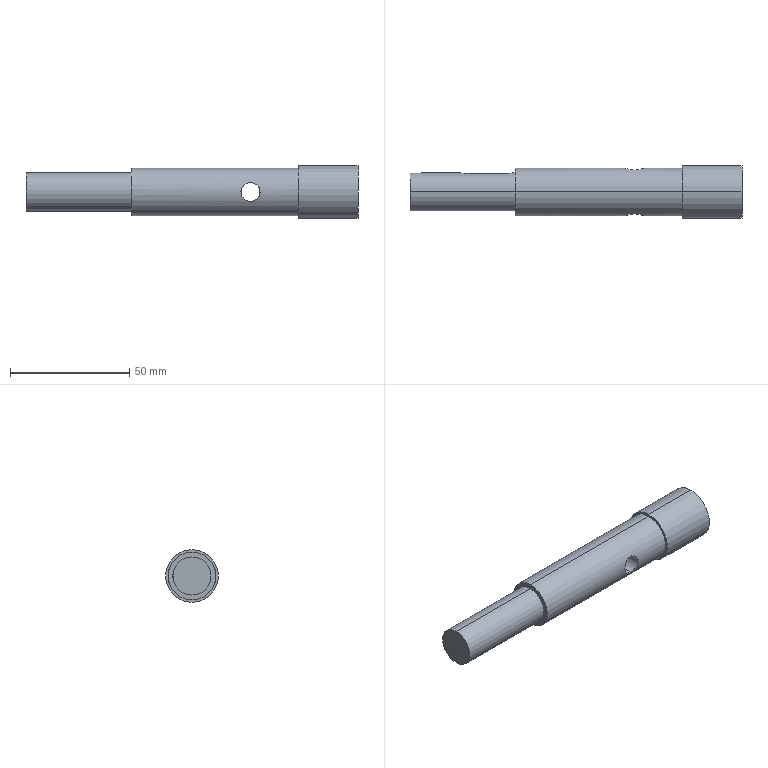Part | SolidWorks | features ICE 2, Revolution 1 | 1 solid | 20 faces | box 139 x 22 x 22 mm | volume 37145 mm3 | cylinder 13 | plane 7 | commonest cylinder face diameters 8 x5 4 x2 16 x2 20 x2 22 x2
STEP:
#1=CARTESIAN_POINT('',(94.,-9.165,-4.));
#2=VERTEX_POINT('',#1);
#3=CARTESIAN_POINT('',(94.,-9.165,4.));
#4=VERTEX_POINT('',#3);
#5=CARTESIAN_POINT('',(94.,-9.165,-4.));
#6=CARTESIAN_POINT('',(93.737,-9.165,-4.));
#7=CARTESIAN_POINT('',(93.471,-9.177,-3.974));
#8=CARTESIAN_POINT('',(92.952,-9.221,-3.869));
#9=CARTESIAN_POINT('',(92.702,-9.254,-3.793));
#10=CARTESIAN_POINT('',(92.219,-9.334,-3.591));
#11=CARTESIAN_POINT('',(91.987,-9.381,-3.466));
#12=CARTESIAN_POINT('',(91.557,-9.483,-3.178));
#13=CARTESIAN_POINT('',(91.356,-9.537,-3.013));
#14=CARTESIAN_POINT('',(90.987,-9.646,-2.644));
#15=CARTESIAN_POINT('',(90.823,-9.699,-2.444));
#16=CARTESIAN_POINT('',(90.535,-9.797,-2.015));
#17=CARTESIAN_POINT('',(90.409,-9.843,-1.782));
#18=CARTESIAN_POINT('',(90.208,-9.918,-1.299));
#19=CARTESIAN_POINT('',(90.131,-9.948,-1.049));
#20=CARTESIAN_POINT('',(90.027,-9.989,-0.5334));
#21=CARTESIAN_POINT('',(90.,-10.,-0.2654));
#22=CARTESIAN_POINT('',(90.,-10.,0.2618));
#23=CARTESIAN_POINT('',(90.026,-9.99,0.5238));
#24=CARTESIAN_POINT('',(90.13,-9.949,1.045));
#25=CARTESIAN_POINT('',(90.207,-9.919,1.297));
#26=CARTESIAN_POINT('',(90.408,-9.843,1.779));
#27=CARTESIAN_POINT('',(90.533,-9.798,2.012));
#28=CARTESIAN_POINT('',(90.823,-9.699,2.444));
#29=CARTESIAN_POINT('',(90.987,-9.646,2.644));
#30=CARTESIAN_POINT('',(91.354,-9.538,3.011));
#31=CARTESIAN_POINT('',(91.557,-9.483,3.177));
#32=CARTESIAN_POINT('',(91.986,-9.382,3.465));
#33=CARTESIAN_POINT('',(92.214,-9.335,3.589));
#34=CARTESIAN_POINT('',(92.7,-9.254,3.792));
#35=CARTESIAN_POINT('',(92.952,-9.221,3.869));
#36=CARTESIAN_POINT('',(93.467,-9.177,3.973));
#37=CARTESIAN_POINT('',(93.733,-9.165,4.));
#38=CARTESIAN_POINT('',(94.,-9.165,4.));
#39=B_SPLINE_CURVE_WITH_KNOTS('',3,(#5,#6,#7,#8,#9,#10,#11,#12,#13,#14,#15,#16,#17,#18,#19,#20,#21,#22,#23,#24,#25,#26,#27,#28,#29,#30,#31,#32,#33,#34,#35,#36,#37,#38),.UNSPECIFIED.,.F.,.F.,(4,2,2,2,2,2,2,2,2,2,2,2,2,2,2,2,4),(0.01264,0.01343,0.01422,0.01501,0.0158,0.01658,0.01737,0.01816,0.01895,0.01974,0.02053,0.02132,0.02211,0.0229,0.02369,0.02448,0.02527),.UNSPECIFIED.);
#40=EDGE_CURVE('',#2,#4,#39,.T.);
#41=ORIENTED_EDGE('',*,*,#40,.F.);
#42=CARTESIAN_POINT('',(94.,0.,-4.));
#43=VERTEX_POINT('',#42);
#44=CARTESIAN_POINT('',(94.,-11.,-4.));
#45=DIRECTION('',(0.,1.,0.));
#46=VECTOR('',#45,1000.);
#47=LINE('',#44,#46);
#48=EDGE_CURVE('',#2,#43,#47,.T.);
#49=ORIENTED_EDGE('',*,*,#48,.T.);
#50=CARTESIAN_POINT('',(94.,9.165,-4.));
#51=VERTEX_POINT('',#50);
#52=CARTESIAN_POINT('',(94.,-11.,-4.));
#53=DIRECTION('',(0.,1.,0.));
#54=VECTOR('',#53,1000.);
#55=LINE('',#52,#54);
#56=EDGE_CURVE('',#43,#51,#55,.T.);
#57=ORIENTED_EDGE('',*,*,#56,.T.);
#58=CARTESIAN_POINT('',(94.,9.165,4.));
#59=VERTEX_POINT('',#58);
#60=CARTESIAN_POINT('',(94.,9.165,4.));
#61=CARTESIAN_POINT('',(93.733,9.165,4.));
#62=CARTESIAN_POINT('',(93.47,9.177,3.973));
#63=CARTESIAN_POINT('',(92.955,9.221,3.87));
#64=CARTESIAN_POINT('',(92.7,9.254,3.792));
#65=CARTESIAN_POINT('',(92.217,9.334,3.59));
#66=CARTESIAN_POINT('',(91.989,9.381,3.467));
#67=CARTESIAN_POINT('',(91.556,9.483,3.177));
#68=CARTESIAN_POINT('',(91.354,9.538,3.011));
#69=CARTESIAN_POINT('',(90.989,9.646,2.646));
#70=CARTESIAN_POINT('',(90.824,9.699,2.445));
#71=CARTESIAN_POINT('',(90.532,9.798,2.01));
#72=CARTESIAN_POINT('',(90.409,9.843,1.781));
#73=CARTESIAN_POINT('',(90.208,9.918,1.301));
#74=CARTESIAN_POINT('',(90.13,9.949,1.046));
#75=CARTESIAN_POINT('',(90.026,9.989,0.5279));
#76=CARTESIAN_POINT('',(90.,10.,0.2663));
#77=CARTESIAN_POINT('',(90.,10.,-0.2622));
#78=CARTESIAN_POINT('',(90.027,9.989,-0.5302));
#79=CARTESIAN_POINT('',(90.13,9.949,-1.046));
#80=CARTESIAN_POINT('',(90.207,9.919,-1.297));
#81=CARTESIAN_POINT('',(90.411,9.842,-1.785));
#82=CARTESIAN_POINT('',(90.534,9.798,-2.014));
#83=CARTESIAN_POINT('',(90.824,9.699,-2.445));
#84=CARTESIAN_POINT('',(90.991,9.645,-2.648));
#85=CARTESIAN_POINT('',(91.358,9.537,-3.014));
#86=CARTESIAN_POINT('',(91.557,9.483,-3.178));
#87=CARTESIAN_POINT('',(91.989,9.381,-3.467));
#88=CARTESIAN_POINT('',(92.222,9.333,-3.592));
#89=CARTESIAN_POINT('',(92.702,9.254,-3.792));
#90=CARTESIAN_POINT('',(92.952,9.221,-3.869));
#91=CARTESIAN_POINT('',(93.473,9.177,-3.974));
#92=CARTESIAN_POINT('',(93.737,9.165,-4.));
#93=CARTESIAN_POINT('',(94.,9.165,-4.));
#94=B_SPLINE_CURVE_WITH_KNOTS('',3,(#60,#61,#62,#63,#64,#65,#66,#67,#68,#69,#70,#71,#72,#73,#74,#75,#76,#77,#78,#79,#80,#81,#82,#83,#84,#85,#86,#87,#88,#89,#90,#91,#92,#93),.UNSPECIFIED.,.F.,.F.,(4,2,2,2,2,2,2,2,2,2,2,2,2,2,2,2,4),(0.,0.0007899,0.00158,0.00237,0.00316,0.00395,0.00474,0.00553,0.006319,0.007109,0.007899,0.008689,0.009479,0.01027,0.01106,0.01185,0.01264),.UNSPECIFIED.);
#95=EDGE_CURVE('',#59,#51,#94,.T.);
#96=ORIENTED_EDGE('',*,*,#95,.F.);
#97=CARTESIAN_POINT('',(94.,0.,4.));
#98=VERTEX_POINT('',#97);
#99=CARTESIAN_POINT('',(94.,-11.,4.));
#100=DIRECTION('',(0.,1.,0.));
#101=VECTOR('',#100,1000.);
#102=LINE('',#99,#101);
#103=EDGE_CURVE('',#98,#59,#102,.T.);
#104=ORIENTED_EDGE('',*,*,#103,.F.);
#105=CARTESIAN_POINT('',(94.,-11.,4.));
#106=DIRECTION('',(0.,1.,0.));
#107=VECTOR('',#106,1000.);
#108=LINE('',#105,#107);
#109=EDGE_CURVE('',#4,#98,#108,.T.);
#110=ORIENTED_EDGE('',*,*,#109,.F.);
#111=EDGE_LOOP('',(#41,#49,#57,#96,#104,#110));
#112=FACE_OUTER_BOUND('',#111,.T.);
#113=CARTESIAN_POINT('',(94.,-11.,0.));
#114=DIRECTION('',(0.,1.,0.));
#115=DIRECTION('',(0.,0.,1.));
#116=AXIS2_PLACEMENT_3D('',#113,#114,#115);
#117=CYLINDRICAL_SURFACE('',#116,4.);
#118=ADVANCED_FACE('',(#112),#117,.F.);
#119=ORIENTED_EDGE('',*,*,#48,.F.);
#120=CARTESIAN_POINT('',(94.,-9.165,4.));
#121=CARTESIAN_POINT('',(94.267,-9.165,4.));
#122=CARTESIAN_POINT('',(94.53,-9.177,3.973));
#123=CARTESIAN_POINT('',(95.045,-9.221,3.87));
#124=CARTESIAN_POINT('',(95.3,-9.254,3.792));
#125=CARTESIAN_POINT('',(95.783,-9.334,3.59));
#126=CARTESIAN_POINT('',(96.011,-9.381,3.467));
#127=CARTESIAN_POINT('',(96.444,-9.483,3.177));
#128=CARTESIAN_POINT('',(96.646,-9.538,3.011));
#129=CARTESIAN_POINT('',(97.011,-9.646,2.646));
#130=CARTESIAN_POINT('',(97.176,-9.699,2.445));
#131=CARTESIAN_POINT('',(97.468,-9.798,2.01));
#132=CARTESIAN_POINT('',(97.591,-9.843,1.781));
#133=CARTESIAN_POINT('',(97.792,-9.918,1.301));
#134=CARTESIAN_POINT('',(97.87,-9.949,1.046));
#135=CARTESIAN_POINT('',(97.974,-9.989,0.5279));
#136=CARTESIAN_POINT('',(98.,-10.,0.2663));
#137=CARTESIAN_POINT('',(98.,-10.,-0.2622));
#138=CARTESIAN_POINT('',(97.973,-9.989,-0.5302));
#139=CARTESIAN_POINT('',(97.87,-9.949,-1.046));
#140=CARTESIAN_POINT('',(97.793,-9.919,-1.297));
#141=CARTESIAN_POINT('',(97.589,-9.842,-1.785));
#142=CARTESIAN_POINT('',(97.466,-9.798,-2.014));
#143=CARTESIAN_POINT('',(97.176,-9.699,-2.445));
#144=CARTESIAN_POINT('',(97.009,-9.645,-2.648));
#145=CARTESIAN_POINT('',(96.642,-9.537,-3.014));
#146=CARTESIAN_POINT('',(96.443,-9.483,-3.178));
#147=CARTESIAN_POINT('',(96.011,-9.381,-3.467));
#148=CARTESIAN_POINT('',(95.778,-9.333,-3.592));
#149=CARTESIAN_POINT('',(95.298,-9.254,-3.792));
#150=CARTESIAN_POINT('',(95.048,-9.221,-3.869));
#151=CARTESIAN_POINT('',(94.527,-9.177,-3.974));
#152=CARTESIAN_POINT('',(94.263,-9.165,-4.));
#153=CARTESIAN_POINT('',(94.,-9.165,-4.));
#154=B_SPLINE_CURVE_WITH_KNOTS('',3,(#120,#121,#122,#123,#124,#125,#126,#127,#128,#129,#130,#131,#132,#133,#134,#135,#136,#137,#138,#139,#140,#141,#142,#143,#144,#145,#146,#147,#148,#149,#150,#151,#152,#153),.UNSPECIFIED.,.F.,.F.,(4,2,2,2,2,2,2,2,2,2,2,2,2,2,2,2,4),(0.,0.0007899,0.00158,0.00237,0.00316,0.00395,0.00474,0.00553,0.006319,0.007109,0.007899,0.008689,0.009479,0.01027,0.01106,0.01185,0.01264),.UNSPECIFIED.);
#155=EDGE_CURVE('',#4,#2,#154,.T.);
#156=ORIENTED_EDGE('',*,*,#155,.F.);
#157=ORIENTED_EDGE('',*,*,#109,.T.);
#158=CARTESIAN_POINT('',(94.,0.,-4.));
#159=CARTESIAN_POINT('',(102.,-8.,-4.));
#160=CARTESIAN_POINT('',(102.,-8.,4.));
#161=CARTESIAN_POINT('',(94.,0.,4.));
#162=(BOUNDED_CURVE()B_SPLINE_CURVE(3,(#158,#159,#160,#161),.UNSPECIFIED.,.F.,.T.)B_SPLINE_CURVE_WITH_KNOTS((4,4),(1.571,4.712),.UNSPECIFIED.)CURVE()GEOMETRIC_REPRESENTATION_ITEM()RATIONAL_B_SPLINE_CURVE((1.,0.3333,0.3333,1.))REPRESENTATION_ITEM(''));
#163=EDGE_CURVE('',#43,#98,#162,.T.);
#164=ORIENTED_EDGE('',*,*,#163,.F.);
#165=EDGE_LOOP('',(#119,#156,#157,#164));
#166=FACE_OUTER_BOUND('',#165,.T.);
#167=CARTESIAN_POINT('',(94.,-11.,0.));
#168=DIRECTION('',(0.,1.,0.));
#169=DIRECTION('',(0.,0.,1.));
#170=AXIS2_PLACEMENT_3D('',#167,#168,#169);
#171=CYLINDRICAL_SURFACE('',#170,4.);
#172=ADVANCED_FACE('',(#166),#171,.F.);
#173=CARTESIAN_POINT('',(139.,0.,-4.));
#174=VERTEX_POINT('',#173);
#175=CARTESIAN_POINT('',(139.,0.,4.));
#176=VERTEX_POINT('',#175);
#177=CARTESIAN_POINT('',(139.,0.,0.));
#178=DIRECTION('',(-1.,0.,0.));
#179=DIRECTION('',(0.,0.,1.));
#180=AXIS2_PLACEMENT_3D('',#177,#178,#179);
#181=CIRCLE('',#180,4.);
#182=EDGE_CURVE('',#174,#176,#181,.T.);
#183=ORIENTED_EDGE('',*,*,#182,.F.);
#184=CARTESIAN_POINT('',(0.,0.,-4.));
#185=DIRECTION('',(-1.,0.,0.));
#186=VECTOR('',#185,1000.);
#187=LINE('',#184,#186);
#188=EDGE_CURVE('',#174,#43,#187,.T.);
#189=ORIENTED_EDGE('',*,*,#188,.T.);
#190=ORIENTED_EDGE('',*,*,#163,.T.);
#191=CARTESIAN_POINT('',(0.,0.,4.));
#192=DIRECTION('',(-1.,0.,0.));
#193=VECTOR('',#192,1000.);
#194=LINE('',#191,#193);
#195=EDGE_CURVE('',#176,#98,#194,.T.);
#196=ORIENTED_EDGE('',*,*,#195,.F.);
#197=EDGE_LOOP('',(#183,#189,#190,#196));
#198=FACE_OUTER_BOUND('',#197,.T.);
#199=CARTESIAN_POINT('',(0.,0.,0.));
#200=DIRECTION('',(-1.,0.,0.));
#201=DIRECTION('',(0.,0.,1.));
#202=AXIS2_PLACEMENT_3D('',#199,#200,#201);
#203=CYLINDRICAL_SURFACE('',#202,4.);
#204=ADVANCED_FACE('',(#198),#203,.F.);
#205=CARTESIAN_POINT('',(139.,0.,11.));
#206=VERTEX_POINT('',#205);
#207=CARTESIAN_POINT('',(139.,0.,-11.));
#208=VERTEX_POINT('',#207);
#209=CARTESIAN_POINT('',(139.,0.,0.));
#210=DIRECTION('',(-1.,0.,0.));
#211=DIRECTION('',(0.,0.,1.));
#212=AXIS2_PLACEMENT_3D('',#209,#210,#211);
#213=CIRCLE('',#212,11.);
#214=EDGE_CURVE('',#206,#208,#213,.T.);
#215=ORIENTED_EDGE('',*,*,#214,.T.);
#216=CARTESIAN_POINT('',(114.,0.,-11.));
#217=VERTEX_POINT('',#216);
#218=CARTESIAN_POINT('',(0.,0.,-11.));
#219=DIRECTION('',(-1.,0.,0.));
#220=VECTOR('',#219,1000.);
#221=LINE('',#218,#220);
#222=EDGE_CURVE('',#208,#217,#221,.T.);
#223=ORIENTED_EDGE('',*,*,#222,.T.);
#224=CARTESIAN_POINT('',(114.,0.,11.));
#225=VERTEX_POINT('',#224);
#226=CARTESIAN_POINT('',(114.,0.,0.));
#227=DIRECTION('',(-1.,0.,0.));
#228=DIRECTION('',(0.,0.,1.));
#229=AXIS2_PLACEMENT_3D('',#226,#227,#228);
#230=CIRCLE('',#229,11.);
#231=EDGE_CURVE('',#225,#217,#230,.T.);
#232=ORIENTED_EDGE('',*,*,#231,.F.);
#233=CARTESIAN_POINT('',(0.,0.,11.));
#234=DIRECTION('',(-1.,0.,0.));
#235=VECTOR('',#234,1000.);
#236=LINE('',#233,#235);
#237=EDGE_CURVE('',#206,#225,#236,.T.);
#238=ORIENTED_EDGE('',*,*,#237,.F.);
#239=EDGE_LOOP('',(#215,#223,#232,#238));
#240=FACE_OUTER_BOUND('',#239,.T.);
#241=CARTESIAN_POINT('',(0.,0.,0.));
#242=DIRECTION('',(-1.,0.,0.));
#243=DIRECTION('',(0.,0.,1.));
#244=AXIS2_PLACEMENT_3D('',#241,#242,#243);
#245=CYLINDRICAL_SURFACE('',#244,11.);
#246=ADVANCED_FACE('',(#240),#245,.T.);
#247=ORIENTED_EDGE('',*,*,#95,.T.);
#248=CARTESIAN_POINT('',(94.,9.165,-4.));
#249=CARTESIAN_POINT('',(94.263,9.165,-4.));
#250=CARTESIAN_POINT('',(94.529,9.177,-3.974));
#251=CARTESIAN_POINT('',(95.048,9.221,-3.869));
#252=CARTESIAN_POINT('',(95.298,9.254,-3.793));
#253=CARTESIAN_POINT('',(95.781,9.334,-3.591));
#254=CARTESIAN_POINT('',(96.013,9.381,-3.466));
#255=CARTESIAN_POINT('',(96.443,9.483,-3.178));
#256=CARTESIAN_POINT('',(96.644,9.537,-3.013));
#257=CARTESIAN_POINT('',(97.013,9.646,-2.644));
#258=CARTESIAN_POINT('',(97.177,9.699,-2.444));
#259=CARTESIAN_POINT('',(97.465,9.797,-2.015));
#260=CARTESIAN_POINT('',(97.591,9.843,-1.782));
#261=CARTESIAN_POINT('',(97.792,9.918,-1.299));
#262=CARTESIAN_POINT('',(97.869,9.948,-1.049));
#263=CARTESIAN_POINT('',(97.973,9.989,-0.5334));
#264=CARTESIAN_POINT('',(98.,10.,-0.2654));
#265=CARTESIAN_POINT('',(98.,10.,0.2618));
#266=CARTESIAN_POINT('',(97.974,9.99,0.5238));
#267=CARTESIAN_POINT('',(97.87,9.949,1.045));
#268=CARTESIAN_POINT('',(97.793,9.919,1.297));
#269=CARTESIAN_POINT('',(97.592,9.843,1.779));
#270=CARTESIAN_POINT('',(97.467,9.798,2.012));
#271=CARTESIAN_POINT('',(97.177,9.699,2.444));
#272=CARTESIAN_POINT('',(97.013,9.646,2.644));
#273=CARTESIAN_POINT('',(96.646,9.538,3.011));
#274=CARTESIAN_POINT('',(96.443,9.483,3.177));
#275=CARTESIAN_POINT('',(96.014,9.382,3.465));
#276=CARTESIAN_POINT('',(95.786,9.335,3.589));
#277=CARTESIAN_POINT('',(95.3,9.254,3.792));
#278=CARTESIAN_POINT('',(95.048,9.221,3.869));
#279=CARTESIAN_POINT('',(94.533,9.177,3.973));
#280=CARTESIAN_POINT('',(94.267,9.165,4.));
#281=CARTESIAN_POINT('',(94.,9.165,4.));
#282=B_SPLINE_CURVE_WITH_KNOTS('',3,(#248,#249,#250,#251,#252,#253,#254,#255,#256,#257,#258,#259,#260,#261,#262,#263,#264,#265,#266,#267,#268,#269,#270,#271,#272,#273,#274,#275,#276,#277,#278,#279,#280,#281),.UNSPECIFIED.,.F.,.F.,(4,2,2,2,2,2,2,2,2,2,2,2,2,2,2,2,4),(0.01264,0.01343,0.01422,0.01501,0.0158,0.01658,0.01737,0.01816,0.01895,0.01974,0.02053,0.02132,0.02211,0.0229,0.02369,0.02448,0.02527),.UNSPECIFIED.);
#283=EDGE_CURVE('',#51,#59,#282,.T.);
#284=ORIENTED_EDGE('',*,*,#283,.T.);
#285=EDGE_LOOP('',(#247,#284));
#286=FACE_BOUND('',#285,.T.);
#287=CARTESIAN_POINT('',(114.,0.,10.));
#288=VERTEX_POINT('',#287);
#289=CARTESIAN_POINT('',(114.,0.,-10.));
#290=VERTEX_POINT('',#289);
#291=CARTESIAN_POINT('',(114.,0.,0.));
#292=DIRECTION('',(-1.,0.,0.));
#293=DIRECTION('',(0.,0.,1.));
#294=AXIS2_PLACEMENT_3D('',#291,#292,#293);
#295=CIRCLE('',#294,10.);
#296=EDGE_CURVE('',#288,#290,#295,.T.);
#297=ORIENTED_EDGE('',*,*,#296,.T.);
#298=CARTESIAN_POINT('',(44.,0.,-10.));
#299=VERTEX_POINT('',#298);
#300=CARTESIAN_POINT('',(0.,0.,-10.));
#301=DIRECTION('',(-1.,0.,0.));
#302=VECTOR('',#301,1000.);
#303=LINE('',#300,#302);
#304=EDGE_CURVE('',#290,#299,#303,.T.);
#305=ORIENTED_EDGE('',*,*,#304,.T.);
#306=CARTESIAN_POINT('',(44.,0.,10.));
#307=VERTEX_POINT('',#306);
#308=CARTESIAN_POINT('',(44.,0.,0.));
#309=DIRECTION('',(-1.,0.,0.));
#310=DIRECTION('',(0.,0.,1.));
#311=AXIS2_PLACEMENT_3D('',#308,#309,#310);
#312=CIRCLE('',#311,10.);
#313=EDGE_CURVE('',#307,#299,#312,.T.);
#314=ORIENTED_EDGE('',*,*,#313,.F.);
#315=CARTESIAN_POINT('',(0.,0.,10.));
#316=DIRECTION('',(-1.,0.,0.));
#317=VECTOR('',#316,1000.);
#318=LINE('',#315,#317);
#319=EDGE_CURVE('',#288,#307,#318,.T.);
#320=ORIENTED_EDGE('',*,*,#319,.F.);
#321=EDGE_LOOP('',(#297,#305,#314,#320));
#322=FACE_OUTER_BOUND('',#321,.T.);
#323=CARTESIAN_POINT('',(0.,0.,0.));
#324=DIRECTION('',(-1.,0.,0.));
#325=DIRECTION('',(0.,0.,1.));
#326=AXIS2_PLACEMENT_3D('',#323,#324,#325);
#327=CYLINDRICAL_SURFACE('',#326,10.);
#328=ADVANCED_FACE('',(#286,#322),#327,.T.);
#329=CARTESIAN_POINT('',(23.,7.746,-2.));
#330=VERTEX_POINT('',#329);
#331=CARTESIAN_POINT('',(41.,7.746,-2.));
#332=VERTEX_POINT('',#331);
#333=CARTESIAN_POINT('',(0.,7.746,-2.));
#334=DIRECTION('',(1.,0.,0.));
#335=VECTOR('',#334,1000.);
#336=LINE('',#333,#335);
#337=EDGE_CURVE('',#330,#332,#336,.T.);
#338=ORIENTED_EDGE('',*,*,#337,.T.);
#339=CARTESIAN_POINT('',(41.,7.746,2.));
#340=VERTEX_POINT('',#339);
#341=CARTESIAN_POINT('',(41.,7.746,-2.));
#342=CARTESIAN_POINT('',(41.133,7.746,-2.));
#343=CARTESIAN_POINT('',(41.263,7.749,-1.987));
#344=CARTESIAN_POINT('',(41.519,7.762,-1.936));
#345=CARTESIAN_POINT('',(41.647,7.772,-1.897));
#346=CARTESIAN_POINT('',(41.888,7.796,-1.797));
#347=CARTESIAN_POINT('',(42.003,7.81,-1.735));
#348=CARTESIAN_POINT('',(42.22,7.841,-1.59));
#349=CARTESIAN_POINT('',(42.322,7.858,-1.506));
#350=CARTESIAN_POINT('',(42.598,7.907,-1.231));
#351=CARTESIAN_POINT('',(42.747,7.94,-1.008));
#352=CARTESIAN_POINT('',(42.897,7.975,-0.6478));
#353=CARTESIAN_POINT('',(42.935,7.984,-0.5212));
#354=CARTESIAN_POINT('',(42.987,7.997,-0.2629));
#355=CARTESIAN_POINT('',(43.,8.,-0.1328));
#356=CARTESIAN_POINT('',(43.,8.,0.1292));
#357=CARTESIAN_POINT('',(42.987,7.997,0.2623));
#358=CARTESIAN_POINT('',(42.936,7.984,0.5192));
#359=CARTESIAN_POINT('',(42.898,7.975,0.6442));
#360=CARTESIAN_POINT('',(42.747,7.94,1.008));
#361=CARTESIAN_POINT('',(42.6,7.907,1.228));
#362=CARTESIAN_POINT('',(42.322,7.857,1.506));
#363=CARTESIAN_POINT('',(42.222,7.841,1.589));
#364=CARTESIAN_POINT('',(42.006,7.81,1.734));
#365=CARTESIAN_POINT('',(41.889,7.796,1.796));
#366=CARTESIAN_POINT('',(41.648,7.772,1.897));
#367=CARTESIAN_POINT('',(41.523,7.763,1.935));
#368=CARTESIAN_POINT('',(41.265,7.749,1.987));
#369=CARTESIAN_POINT('',(41.133,7.746,2.));
#370=CARTESIAN_POINT('',(41.,7.746,2.));
#371=B_SPLINE_CURVE_WITH_KNOTS('',3,(#341,#342,#343,#344,#345,#346,#347,#348,#349,#350,#351,#352,#353,#354,#355,#356,#357,#358,#359,#360,#361,#362,#363,#364,#365,#366,#367,#368,#369,#370),.UNSPECIFIED.,.F.,.F.,(4,2,2,2,2,2,2,2,2,2,2,2,2,2,4),(0.,0.0003922,0.0007845,0.001177,0.001569,0.002353,0.002746,0.003138,0.00353,0.003922,0.004707,0.005099,0.005491,0.005884,0.006276),.UNSPECIFIED.);
#372=EDGE_CURVE('',#332,#340,#371,.T.);
#373=ORIENTED_EDGE('',*,*,#372,.T.);
#374=CARTESIAN_POINT('',(23.,7.746,2.));
#375=VERTEX_POINT('',#374);
#376=CARTESIAN_POINT('',(0.,7.746,2.));
#377=DIRECTION('',(-1.,0.,0.));
#378=VECTOR('',#377,1000.);
#379=LINE('',#376,#378);
#380=EDGE_CURVE('',#340,#375,#379,.T.);
#381=ORIENTED_EDGE('',*,*,#380,.T.);
#382=CARTESIAN_POINT('',(23.,7.746,2.));
#383=CARTESIAN_POINT('',(22.867,7.746,2.));
#384=CARTESIAN_POINT('',(22.737,7.749,1.987));
#385=CARTESIAN_POINT('',(22.481,7.762,1.936));
#386=CARTESIAN_POINT('',(22.353,7.772,1.897));
#387=CARTESIAN_POINT('',(22.112,7.796,1.797));
#388=CARTESIAN_POINT('',(21.997,7.81,1.735));
#389=CARTESIAN_POINT('',(21.78,7.841,1.59));
#390=CARTESIAN_POINT('',(21.678,7.858,1.506));
#391=CARTESIAN_POINT('',(21.402,7.907,1.231));
#392=CARTESIAN_POINT('',(21.253,7.94,1.008));
#393=CARTESIAN_POINT('',(21.103,7.975,0.6478));
#394=CARTESIAN_POINT('',(21.065,7.984,0.5212));
#395=CARTESIAN_POINT('',(21.013,7.997,0.2629));
#396=CARTESIAN_POINT('',(21.,8.,0.1328));
#397=CARTESIAN_POINT('',(21.,8.,-0.1292));
#398=CARTESIAN_POINT('',(21.013,7.997,-0.2623));
#399=CARTESIAN_POINT('',(21.064,7.984,-0.5192));
#400=CARTESIAN_POINT('',(21.102,7.975,-0.6442));
#401=CARTESIAN_POINT('',(21.253,7.94,-1.008));
#402=CARTESIAN_POINT('',(21.4,7.907,-1.228));
#403=CARTESIAN_POINT('',(21.678,7.857,-1.506));
#404=CARTESIAN_POINT('',(21.778,7.841,-1.589));
#405=CARTESIAN_POINT('',(21.994,7.81,-1.734));
#406=CARTESIAN_POINT('',(22.111,7.796,-1.796));
#407=CARTESIAN_POINT('',(22.352,7.772,-1.897));
#408=CARTESIAN_POINT('',(22.477,7.763,-1.935));
#409=CARTESIAN_POINT('',(22.735,7.749,-1.987));
#410=CARTESIAN_POINT('',(22.867,7.746,-2.));
#411=CARTESIAN_POINT('',(23.,7.746,-2.));
#412=B_SPLINE_CURVE_WITH_KNOTS('',3,(#382,#383,#384,#385,#386,#387,#388,#389,#390,#391,#392,#393,#394,#395,#396,#397,#398,#399,#400,#401,#402,#403,#404,#405,#406,#407,#408,#409,#410,#411),.UNSPECIFIED.,.F.,.F.,(4,2,2,2,2,2,2,2,2,2,2,2,2,2,4),(0.,0.0003922,0.0007845,0.001177,0.001569,0.002353,0.002746,0.003138,0.00353,0.003922,0.004707,0.005099,0.005491,0.005884,0.006276),.UNSPECIFIED.);
#413=EDGE_CURVE('',#375,#330,#412,.T.);
#414=ORIENTED_EDGE('',*,*,#413,.T.);
#415=EDGE_LOOP('',(#338,#373,#381,#414));
#416=FACE_BOUND('',#415,.T.);
#417=CARTESIAN_POINT('',(44.,0.,8.));
#418=VERTEX_POINT('',#417);
#419=CARTESIAN_POINT('',(44.,0.,-8.));
#420=VERTEX_POINT('',#419);
#421=CARTESIAN_POINT('',(44.,0.,0.));
#422=DIRECTION('',(-1.,0.,0.));
#423=DIRECTION('',(0.,0.,1.));
#424=AXIS2_PLACEMENT_3D('',#421,#422,#423);
#425=CIRCLE('',#424,8.);
#426=EDGE_CURVE('',#418,#420,#425,.T.);
#427=ORIENTED_EDGE('',*,*,#426,.T.);
#428=CARTESIAN_POINT('',(0.,0.,-8.));
#429=VERTEX_POINT('',#428);
#430=CARTESIAN_POINT('',(0.,0.,-8.));
#431=DIRECTION('',(-1.,0.,0.));
#432=VECTOR('',#431,1000.);
#433=LINE('',#430,#432);
#434=EDGE_CURVE('',#420,#429,#433,.T.);
#435=ORIENTED_EDGE('',*,*,#434,.T.);
#436=CARTESIAN_POINT('',(0.,0.,8.));
#437=VERTEX_POINT('',#436);
#438=CARTESIAN_POINT('',(0.,0.,0.));
#439=DIRECTION('',(-1.,0.,0.));
#440=DIRECTION('',(0.,0.,1.));
#441=AXIS2_PLACEMENT_3D('',#438,#439,#440);
#442=CIRCLE('',#441,8.);
#443=EDGE_CURVE('',#437,#429,#442,.T.);
#444=ORIENTED_EDGE('',*,*,#443,.F.);
#445=CARTESIAN_POINT('',(0.,0.,8.));
#446=DIRECTION('',(-1.,0.,0.));
#447=VECTOR('',#446,1000.);
#448=LINE('',#445,#447);
#449=EDGE_CURVE('',#418,#437,#448,.T.);
#450=ORIENTED_EDGE('',*,*,#449,.F.);
#451=EDGE_LOOP('',(#427,#435,#444,#450));
#452=FACE_OUTER_BOUND('',#451,.T.);
#453=CARTESIAN_POINT('',(0.,0.,0.));
#454=DIRECTION('',(-1.,0.,0.));
#455=DIRECTION('',(0.,0.,1.));
#456=AXIS2_PLACEMENT_3D('',#453,#454,#455);
#457=CYLINDRICAL_SURFACE('',#456,8.);
#458=ADVANCED_FACE('',(#416,#452),#457,.T.);
#459=ORIENTED_EDGE('',*,*,#443,.T.);
#460=CARTESIAN_POINT('',(0.,0.,0.));
#461=DIRECTION('',(-1.,0.,0.));
#462=DIRECTION('',(0.,0.,1.));
#463=AXIS2_PLACEMENT_3D('',#460,#461,#462);
#464=CIRCLE('',#463,8.);
#465=EDGE_CURVE('',#429,#437,#464,.T.);
#466=ORIENTED_EDGE('',*,*,#465,.T.);
#467=EDGE_LOOP('',(#459,#466));
#468=FACE_OUTER_BOUND('',#467,.T.);
#469=CARTESIAN_POINT('',(0.,8.,0.));
#470=DIRECTION('',(1.,0.,0.));
#471=DIRECTION('',(0.,0.,-1.));
#472=AXIS2_PLACEMENT_3D('',#469,#470,#471);
#473=PLANE('',#472);
#474=ADVANCED_FACE('',(#468),#473,.F.);
#475=ORIENTED_EDGE('',*,*,#434,.F.);
#476=CARTESIAN_POINT('',(44.,0.,0.));
#477=DIRECTION('',(-1.,0.,0.));
#478=DIRECTION('',(0.,0.,1.));
#479=AXIS2_PLACEMENT_3D('',#476,#477,#478);
#480=CIRCLE('',#479,8.);
#481=EDGE_CURVE('',#420,#418,#480,.T.);
#482=ORIENTED_EDGE('',*,*,#481,.T.);
#483=ORIENTED_EDGE('',*,*,#449,.T.);
#484=ORIENTED_EDGE('',*,*,#465,.F.);
#485=EDGE_LOOP('',(#475,#482,#483,#484));
#486=FACE_OUTER_BOUND('',#485,.T.);
#487=CARTESIAN_POINT('',(0.,0.,0.));
#488=DIRECTION('',(-1.,0.,0.));
#489=DIRECTION('',(0.,0.,1.));
#490=AXIS2_PLACEMENT_3D('',#487,#488,#489);
#491=CYLINDRICAL_SURFACE('',#490,8.);
#492=ADVANCED_FACE('',(#486),#491,.T.);
#493=ORIENTED_EDGE('',*,*,#426,.F.);
#494=ORIENTED_EDGE('',*,*,#481,.F.);
#495=EDGE_LOOP('',(#493,#494));
#496=FACE_BOUND('',#495,.T.);
#497=ORIENTED_EDGE('',*,*,#313,.T.);
#498=CARTESIAN_POINT('',(44.,0.,0.));
#499=DIRECTION('',(-1.,0.,0.));
#500=DIRECTION('',(0.,0.,1.));
#501=AXIS2_PLACEMENT_3D('',#498,#499,#500);
#502=CIRCLE('',#501,10.);
#503=EDGE_CURVE('',#299,#307,#502,.T.);
#504=ORIENTED_EDGE('',*,*,#503,.T.);
#505=EDGE_LOOP('',(#497,#504));
#506=FACE_OUTER_BOUND('',#505,.T.);
#507=CARTESIAN_POINT('',(44.,8.,0.));
#508=DIRECTION('',(1.,0.,0.));
#509=DIRECTION('',(0.,0.,-1.));
#510=AXIS2_PLACEMENT_3D('',#507,#508,#509);
#511=PLANE('',#510);
#512=ADVANCED_FACE('',(#496,#506),#511,.F.);
#513=ORIENTED_EDGE('',*,*,#304,.F.);
#514=CARTESIAN_POINT('',(114.,0.,0.));
#515=DIRECTION('',(-1.,0.,0.));
#516=DIRECTION('',(0.,0.,1.));
#517=AXIS2_PLACEMENT_3D('',#514,#515,#516);
#518=CIRCLE('',#517,10.);
#519=EDGE_CURVE('',#290,#288,#518,.T.);
#520=ORIENTED_EDGE('',*,*,#519,.T.);
#521=ORIENTED_EDGE('',*,*,#319,.T.);
#522=ORIENTED_EDGE('',*,*,#503,.F.);
#523=EDGE_LOOP('',(#513,#520,#521,#522));
#524=FACE_OUTER_BOUND('',#523,.T.);
#525=ORIENTED_EDGE('',*,*,#155,.T.);
#526=ORIENTED_EDGE('',*,*,#40,.T.);
#527=EDGE_LOOP('',(#525,#526));
#528=FACE_BOUND('',#527,.T.);
#529=CARTESIAN_POINT('',(0.,0.,0.));
#530=DIRECTION('',(-1.,0.,0.));
#531=DIRECTION('',(0.,0.,1.));
#532=AXIS2_PLACEMENT_3D('',#529,#530,#531);
#533=CYLINDRICAL_SURFACE('',#532,10.);
#534=ADVANCED_FACE('',(#524,#528),#533,.T.);
#535=ORIENTED_EDGE('',*,*,#296,.F.);
#536=ORIENTED_EDGE('',*,*,#519,.F.);
#537=EDGE_LOOP('',(#535,#536));
#538=FACE_BOUND('',#537,.T.);
#539=ORIENTED_EDGE('',*,*,#231,.T.);
#540=CARTESIAN_POINT('',(114.,0.,0.));
#541=DIRECTION('',(-1.,0.,0.));
#542=DIRECTION('',(0.,0.,1.));
#543=AXIS2_PLACEMENT_3D('',#540,#541,#542);
#544=CIRCLE('',#543,11.);
#545=EDGE_CURVE('',#217,#225,#544,.T.);
#546=ORIENTED_EDGE('',*,*,#545,.T.);
#547=EDGE_LOOP('',(#539,#546));
#548=FACE_OUTER_BOUND('',#547,.T.);
#549=CARTESIAN_POINT('',(114.,10.,0.));
#550=DIRECTION('',(1.,0.,0.));
#551=DIRECTION('',(0.,0.,-1.));
#552=AXIS2_PLACEMENT_3D('',#549,#550,#551);
#553=PLANE('',#552);
#554=ADVANCED_FACE('',(#538,#548),#553,.F.);
#555=ORIENTED_EDGE('',*,*,#222,.F.);
#556=CARTESIAN_POINT('',(139.,0.,0.));
#557=DIRECTION('',(-1.,0.,0.));
#558=DIRECTION('',(0.,0.,1.));
#559=AXIS2_PLACEMENT_3D('',#556,#557,#558);
#560=CIRCLE('',#559,11.);
#561=EDGE_CURVE('',#208,#206,#560,.T.);
#562=ORIENTED_EDGE('',*,*,#561,.T.);
#563=ORIENTED_EDGE('',*,*,#237,.T.);
#564=ORIENTED_EDGE('',*,*,#545,.F.);
#565=EDGE_LOOP('',(#555,#562,#563,#564));
#566=FACE_OUTER_BOUND('',#565,.T.);
#567=CARTESIAN_POINT('',(0.,0.,0.));
#568=DIRECTION('',(-1.,0.,0.));
#569=DIRECTION('',(0.,0.,1.));
#570=AXIS2_PLACEMENT_3D('',#567,#568,#569);
#571=CYLINDRICAL_SURFACE('',#570,11.);
#572=ADVANCED_FACE('',(#566),#571,.T.);
#573=ORIENTED_EDGE('',*,*,#214,.F.);
#574=ORIENTED_EDGE('',*,*,#561,.F.);
#575=EDGE_LOOP('',(#573,#574));
#576=FACE_OUTER_BOUND('',#575,.T.);
#577=CARTESIAN_POINT('',(139.,0.,0.));
#578=DIRECTION('',(-1.,0.,0.));
#579=DIRECTION('',(0.,0.,1.));
#580=AXIS2_PLACEMENT_3D('',#577,#578,#579);
#581=CIRCLE('',#580,4.);
#582=EDGE_CURVE('',#176,#174,#581,.T.);
#583=ORIENTED_EDGE('',*,*,#582,.T.);
#584=ORIENTED_EDGE('',*,*,#182,.T.);
#585=EDGE_LOOP('',(#583,#584));
#586=FACE_BOUND('',#585,.T.);
#587=CARTESIAN_POINT('',(139.,11.,0.));
#588=DIRECTION('',(-1.,0.,0.));
#589=DIRECTION('',(0.,0.,1.));
#590=AXIS2_PLACEMENT_3D('',#587,#588,#589);
#591=PLANE('',#590);
#592=ADVANCED_FACE('',(#576,#586),#591,.F.);
#593=ORIENTED_EDGE('',*,*,#188,.F.);
#594=ORIENTED_EDGE('',*,*,#582,.F.);
#595=ORIENTED_EDGE('',*,*,#195,.T.);
#596=CARTESIAN_POINT('',(94.,0.,4.));
#597=CARTESIAN_POINT('',(102.,8.,4.));
#598=CARTESIAN_POINT('',(102.,8.,-4.));
#599=CARTESIAN_POINT('',(94.,0.,-4.));
#600=(BOUNDED_CURVE()B_SPLINE_CURVE(3,(#596,#597,#598,#599),.UNSPECIFIED.,.F.,.T.)B_SPLINE_CURVE_WITH_KNOTS((4,4),(1.571,4.712),.UNSPECIFIED.)CURVE()GEOMETRIC_REPRESENTATION_ITEM()RATIONAL_B_SPLINE_CURVE((1.,0.3333,0.3333,1.))REPRESENTATION_ITEM(''));
#601=EDGE_CURVE('',#98,#43,#600,.T.);
#602=ORIENTED_EDGE('',*,*,#601,.T.);
#603=EDGE_LOOP('',(#593,#594,#595,#602));
#604=FACE_OUTER_BOUND('',#603,.T.);
#605=CARTESIAN_POINT('',(0.,0.,0.));
#606=DIRECTION('',(-1.,0.,0.));
#607=DIRECTION('',(0.,0.,1.));
#608=AXIS2_PLACEMENT_3D('',#605,#606,#607);
#609=CYLINDRICAL_SURFACE('',#608,4.);
#610=ADVANCED_FACE('',(#604),#609,.F.);
#611=CARTESIAN_POINT('',(23.,6.5,2.));
#612=VERTEX_POINT('',#611);
#613=CARTESIAN_POINT('',(23.,6.5,2.));
#614=DIRECTION('',(0.,1.,0.));
#615=VECTOR('',#614,1000.);
#616=LINE('',#613,#615);
#617=EDGE_CURVE('',#612,#375,#616,.T.);
#618=ORIENTED_EDGE('',*,*,#617,.F.);
#619=CARTESIAN_POINT('',(23.,6.5,-2.));
#620=VERTEX_POINT('',#619);
#621=CARTESIAN_POINT('',(23.,6.5,0.));
#622=DIRECTION('',(0.,1.,0.));
#623=DIRECTION('',(0.,0.,1.));
#624=AXIS2_PLACEMENT_3D('',#621,#622,#623);
#625=CIRCLE('',#624,2.);
#626=EDGE_CURVE('',#620,#612,#625,.T.);
#627=ORIENTED_EDGE('',*,*,#626,.F.);
#628=CARTESIAN_POINT('',(23.,6.5,-2.));
#629=DIRECTION('',(0.,1.,0.));
#630=VECTOR('',#629,1000.);
#631=LINE('',#628,#630);
#632=EDGE_CURVE('',#620,#330,#631,.T.);
#633=ORIENTED_EDGE('',*,*,#632,.T.);
#634=ORIENTED_EDGE('',*,*,#413,.F.);
#635=EDGE_LOOP('',(#618,#627,#633,#634));
#636=FACE_OUTER_BOUND('',#635,.T.);
#637=CARTESIAN_POINT('',(23.,6.5,0.));
#638=DIRECTION('',(0.,1.,0.));
#639=DIRECTION('',(0.,0.,1.));
#640=AXIS2_PLACEMENT_3D('',#637,#638,#639);
#641=CYLINDRICAL_SURFACE('',#640,2.);
#642=ADVANCED_FACE('',(#636),#641,.F.);
#643=ORIENTED_EDGE('',*,*,#632,.F.);
#644=CARTESIAN_POINT('',(41.,6.5,-2.));
#645=VERTEX_POINT('',#644);
#646=CARTESIAN_POINT('',(23.,6.5,-2.));
#647=DIRECTION('',(-1.,0.,0.));
#648=VECTOR('',#647,1000.);
#649=LINE('',#646,#648);
#650=EDGE_CURVE('',#645,#620,#649,.T.);
#651=ORIENTED_EDGE('',*,*,#650,.F.);
#652=CARTESIAN_POINT('',(41.,6.5,-2.));
#653=DIRECTION('',(0.,1.,0.));
#654=VECTOR('',#653,1000.);
#655=LINE('',#652,#654);
#656=EDGE_CURVE('',#645,#332,#655,.T.);
#657=ORIENTED_EDGE('',*,*,#656,.T.);
#658=ORIENTED_EDGE('',*,*,#337,.F.);
#659=EDGE_LOOP('',(#643,#651,#657,#658));
#660=FACE_OUTER_BOUND('',#659,.T.);
#661=CARTESIAN_POINT('',(23.,6.5,-2.));
#662=DIRECTION('',(0.,0.,-1.));
#663=DIRECTION('',(-1.,0.,0.));
#664=AXIS2_PLACEMENT_3D('',#661,#662,#663);
#665=PLANE('',#664);
#666=ADVANCED_FACE('',(#660),#665,.F.);
#667=ORIENTED_EDGE('',*,*,#656,.F.);
#668=CARTESIAN_POINT('',(41.,6.5,2.));
#669=VERTEX_POINT('',#668);
#670=CARTESIAN_POINT('',(41.,6.5,0.));
#671=DIRECTION('',(0.,1.,0.));
#672=DIRECTION('',(0.,0.,1.));
#673=AXIS2_PLACEMENT_3D('',#670,#671,#672);
#674=CIRCLE('',#673,2.);
#675=EDGE_CURVE('',#669,#645,#674,.T.);
#676=ORIENTED_EDGE('',*,*,#675,.F.);
#677=CARTESIAN_POINT('',(41.,6.5,2.));
#678=DIRECTION('',(0.,1.,0.));
#679=VECTOR('',#678,1000.);
#680=LINE('',#677,#679);
#681=EDGE_CURVE('',#669,#340,#680,.T.);
#682=ORIENTED_EDGE('',*,*,#681,.T.);
#683=ORIENTED_EDGE('',*,*,#372,.F.);
#684=EDGE_LOOP('',(#667,#676,#682,#683));
#685=FACE_OUTER_BOUND('',#684,.T.);
#686=CARTESIAN_POINT('',(41.,6.5,0.));
#687=DIRECTION('',(0.,1.,0.));
#688=DIRECTION('',(0.,0.,1.));
#689=AXIS2_PLACEMENT_3D('',#686,#687,#688);
#690=CYLINDRICAL_SURFACE('',#689,2.);
#691=ADVANCED_FACE('',(#685),#690,.F.);
#692=ORIENTED_EDGE('',*,*,#681,.F.);
#693=CARTESIAN_POINT('',(23.,6.5,2.));
#694=DIRECTION('',(1.,0.,0.));
#695=VECTOR('',#694,1000.);
#696=LINE('',#693,#695);
#697=EDGE_CURVE('',#612,#669,#696,.T.);
#698=ORIENTED_EDGE('',*,*,#697,.F.);
#699=ORIENTED_EDGE('',*,*,#617,.T.);
#700=ORIENTED_EDGE('',*,*,#380,.F.);
#701=EDGE_LOOP('',(#692,#698,#699,#700));
#702=FACE_OUTER_BOUND('',#701,.T.);
#703=CARTESIAN_POINT('',(23.,6.5,2.));
#704=DIRECTION('',(0.,0.,1.));
#705=DIRECTION('',(1.,0.,0.));
#706=AXIS2_PLACEMENT_3D('',#703,#704,#705);
#707=PLANE('',#706);
#708=ADVANCED_FACE('',(#702),#707,.F.);
#709=ORIENTED_EDGE('',*,*,#626,.T.);
#710=ORIENTED_EDGE('',*,*,#697,.T.);
#711=ORIENTED_EDGE('',*,*,#675,.T.);
#712=ORIENTED_EDGE('',*,*,#650,.T.);
#713=EDGE_LOOP('',(#709,#710,#711,#712));
#714=FACE_OUTER_BOUND('',#713,.T.);
#715=CARTESIAN_POINT('',(23.,6.5,0.));
#716=DIRECTION('',(0.,1.,0.));
#717=DIRECTION('',(0.,0.,1.));
#718=AXIS2_PLACEMENT_3D('',#715,#716,#717);
#719=PLANE('',#718);
#720=ADVANCED_FACE('',(#714),#719,.T.);
#721=ORIENTED_EDGE('',*,*,#56,.F.);
#722=ORIENTED_EDGE('',*,*,#601,.F.);
#723=ORIENTED_EDGE('',*,*,#103,.T.);
#724=ORIENTED_EDGE('',*,*,#283,.F.);
#725=EDGE_LOOP('',(#721,#722,#723,#724));
#726=FACE_OUTER_BOUND('',#725,.T.);
#727=CARTESIAN_POINT('',(94.,-11.,0.));
#728=DIRECTION('',(0.,1.,0.));
#729=DIRECTION('',(0.,0.,1.));
#730=AXIS2_PLACEMENT_3D('',#727,#728,#729);
#731=CYLINDRICAL_SURFACE('',#730,4.);
#732=ADVANCED_FACE('',(#726),#731,.F.);
#733=CLOSED_SHELL('',(#118,#172,#204,#246,#328,#458,#474,#492,#512,#534,#554,#572,#592,#610,#642,#666,#691,#708,#720,#732));
#734=MANIFOLD_SOLID_BREP('',#733);
#735=CARTESIAN_POINT('',(0.,0.,0.));
#736=DIRECTION('',(0.,0.,1.));
#737=DIRECTION('',(1.,0.,0.));
#738=AXIS2_PLACEMENT_3D('',#735,#736,#737);
#739=(LENGTH_UNIT()NAMED_UNIT(*)SI_UNIT(.MILLI.,.METRE.));
#740=UNCERTAINTY_MEASURE_WITH_UNIT(LENGTH_MEASURE(0.00001),#739,'','');
#741=(NAMED_UNIT(*)PLANE_ANGLE_UNIT()SI_UNIT($,.RADIAN.));
#742=(NAMED_UNIT(*)SI_UNIT($,.STERADIAN.)SOLID_ANGLE_UNIT());
#743=(GEOMETRIC_REPRESENTATION_CONTEXT(3)GLOBAL_UNCERTAINTY_ASSIGNED_CONTEXT((#740))GLOBAL_UNIT_ASSIGNED_CONTEXT((#739,#741,#742))REPRESENTATION_CONTEXT('',''));
#744=ADVANCED_BREP_SHAPE_REPRESENTATION('',(#734,#738),#743);